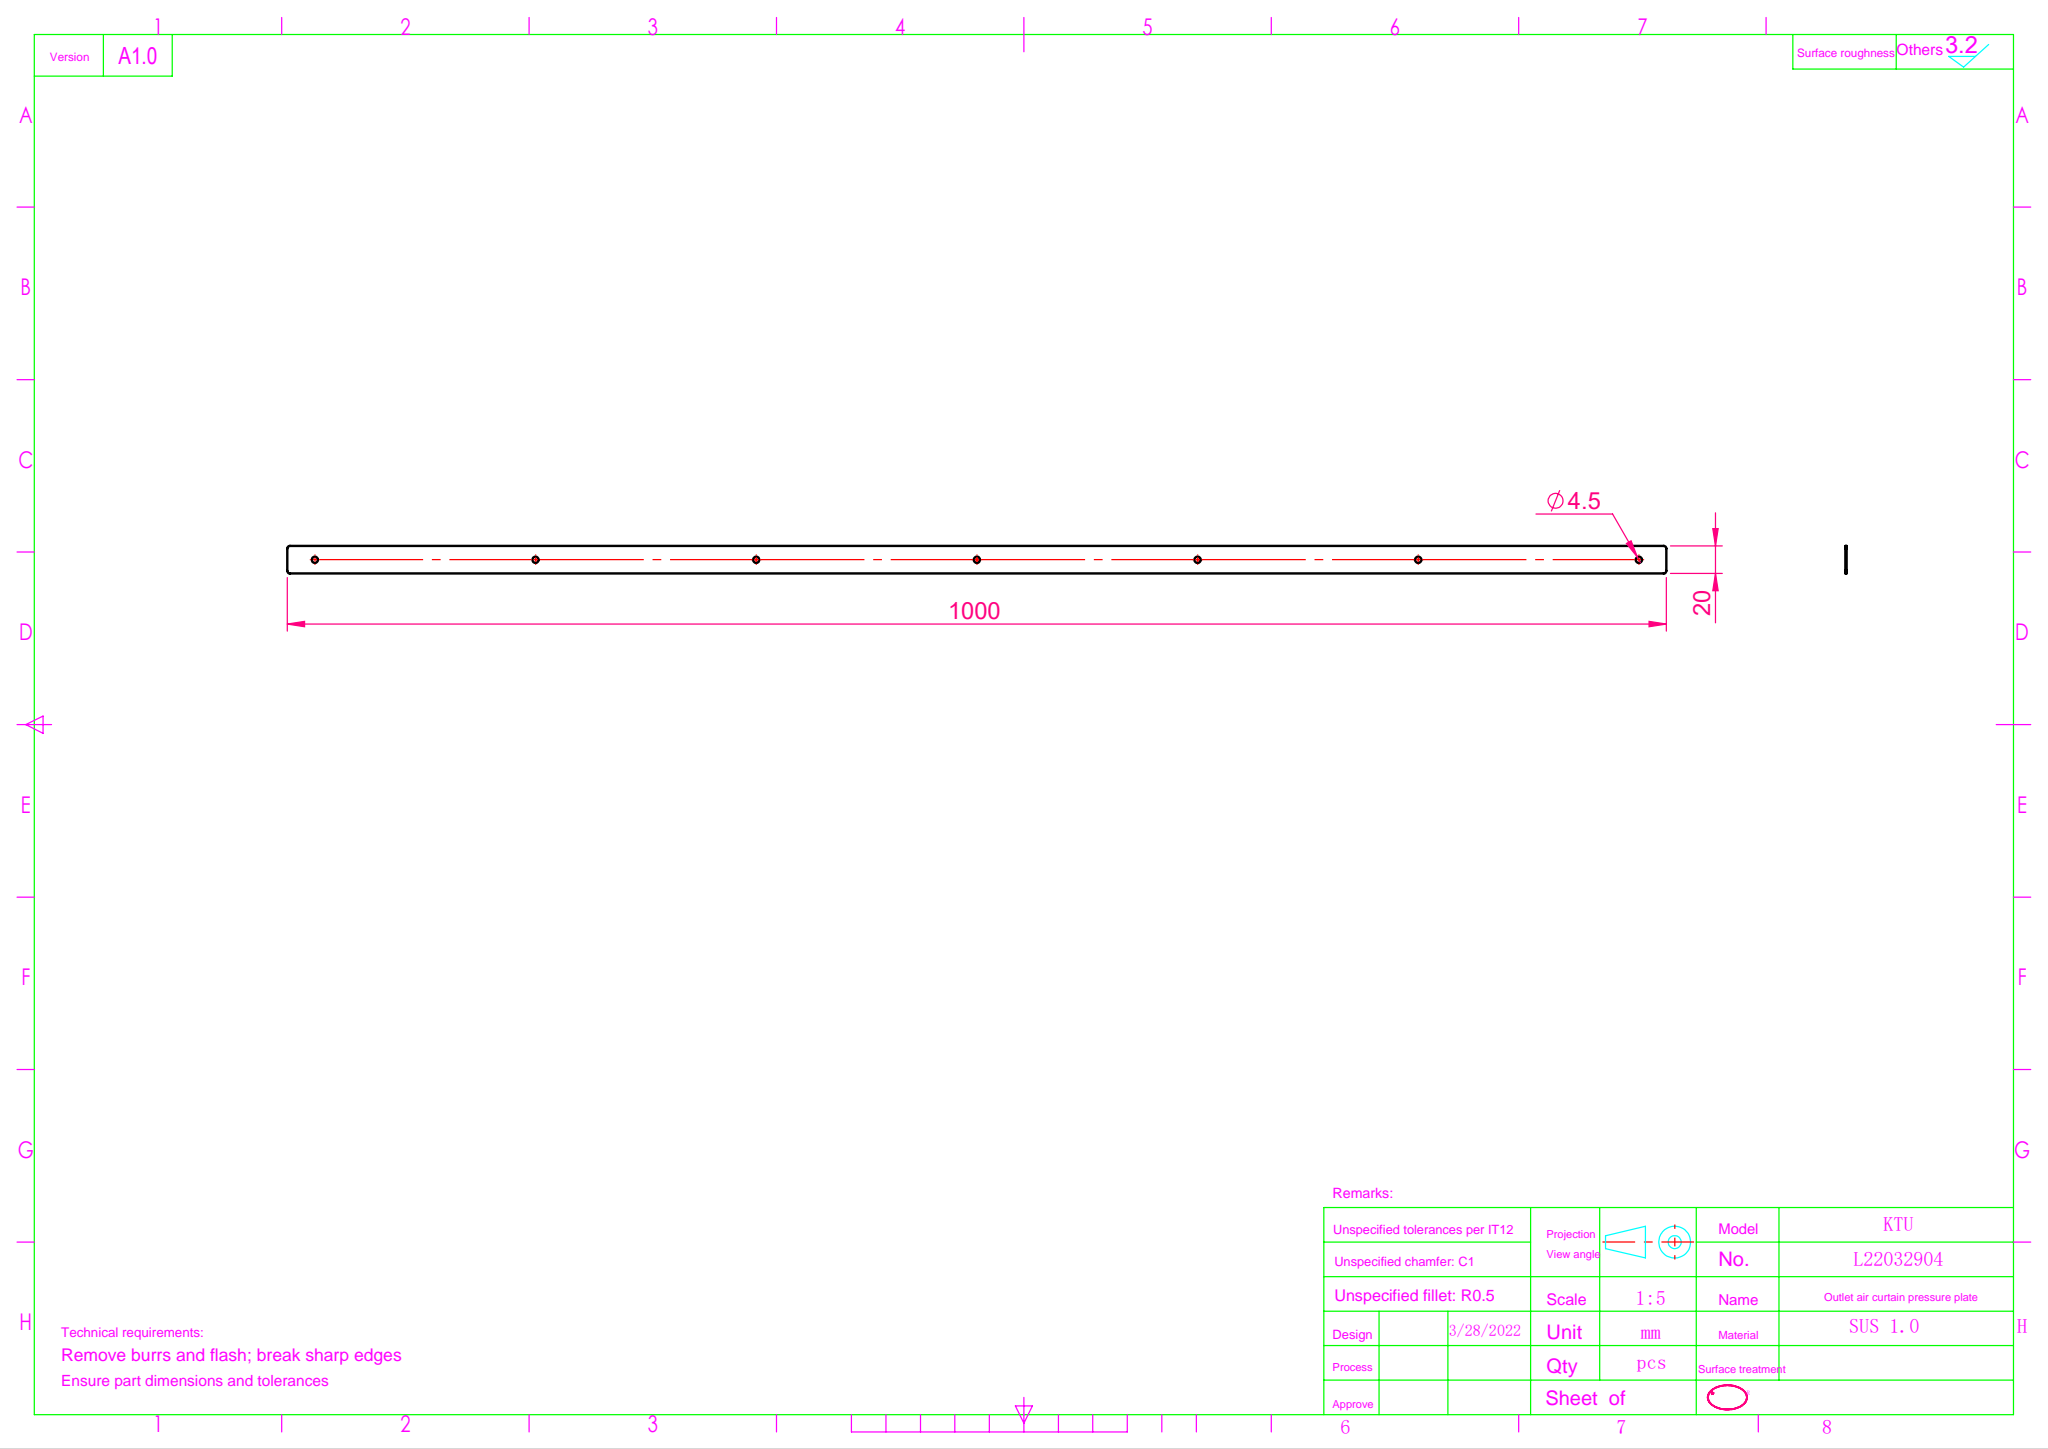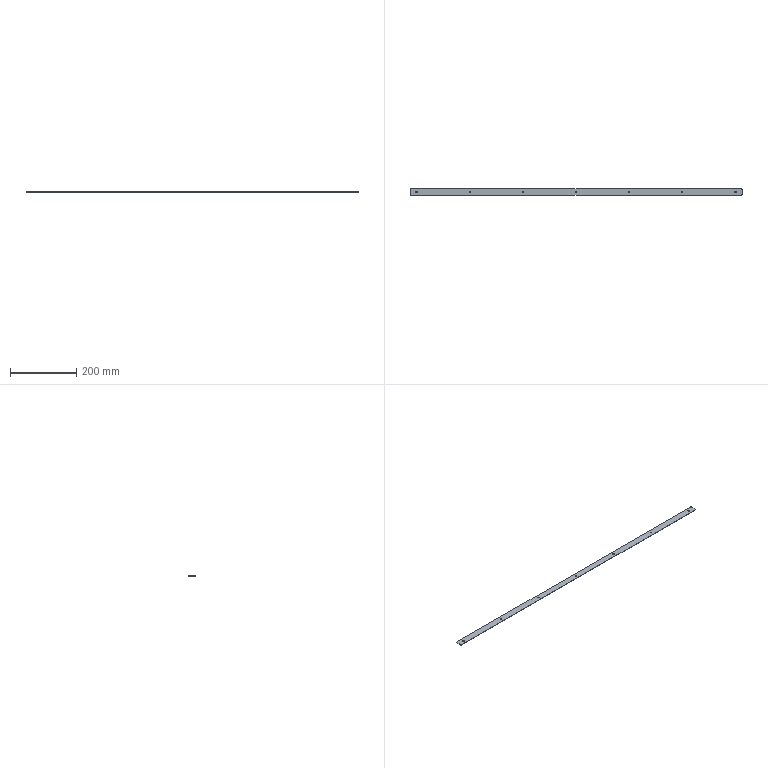Part | SolidWorks | features Fillet 1, FlatPattern 1, ICE 1, LPattern 1, SMBaseFlange 1, SheetMetal 1 | 1 solid | 24 faces | box 1000 x 20 x 1 mm | volume 19885 mm3 | cylinder 18 | plane 6 | commonest cylinder face diameters 4.5 x14 4 x4
STEP:
#1=CARTESIAN_POINT('',(-322.25,0.,-1.));
#2=VERTEX_POINT('',#1);
#3=CARTESIAN_POINT('',(-317.75,0.,-1.));
#4=VERTEX_POINT('',#3);
#5=CARTESIAN_POINT('',(-320.,0.,-1.));
#6=DIRECTION('',(0.,0.,1.));
#7=DIRECTION('',(1.,0.,0.));
#8=AXIS2_PLACEMENT_3D('',#5,#6,#7);
#9=CIRCLE('',#8,2.25);
#10=EDGE_CURVE('',#2,#4,#9,.T.);
#11=ORIENTED_EDGE('',*,*,#10,.F.);
#12=CARTESIAN_POINT('',(-322.25,0.,0.));
#13=VERTEX_POINT('',#12);
#14=CARTESIAN_POINT('',(-322.25,0.,-1.));
#15=DIRECTION('',(0.,0.,1.));
#16=VECTOR('',#15,1000.);
#17=LINE('',#14,#16);
#18=EDGE_CURVE('',#2,#13,#17,.T.);
#19=ORIENTED_EDGE('',*,*,#18,.T.);
#20=CARTESIAN_POINT('',(-317.75,0.,0.));
#21=VERTEX_POINT('',#20);
#22=CARTESIAN_POINT('',(-320.,0.,0.));
#23=DIRECTION('',(0.,0.,1.));
#24=DIRECTION('',(1.,0.,0.));
#25=AXIS2_PLACEMENT_3D('',#22,#23,#24);
#26=CIRCLE('',#25,2.25);
#27=EDGE_CURVE('',#13,#21,#26,.T.);
#28=ORIENTED_EDGE('',*,*,#27,.T.);
#29=CARTESIAN_POINT('',(-317.75,0.,-1.));
#30=DIRECTION('',(0.,0.,1.));
#31=VECTOR('',#30,1000.);
#32=LINE('',#29,#31);
#33=EDGE_CURVE('',#4,#21,#32,.T.);
#34=ORIENTED_EDGE('',*,*,#33,.F.);
#35=EDGE_LOOP('',(#11,#19,#28,#34));
#36=FACE_OUTER_BOUND('',#35,.T.);
#37=CARTESIAN_POINT('',(-320.,0.,-1.));
#38=DIRECTION('',(0.,0.,1.));
#39=DIRECTION('',(1.,0.,0.));
#40=AXIS2_PLACEMENT_3D('',#37,#38,#39);
#41=CYLINDRICAL_SURFACE('',#40,2.25);
#42=ADVANCED_FACE('',(#36),#41,.F.);
#43=CARTESIAN_POINT('',(317.75,0.,-1.));
#44=VERTEX_POINT('',#43);
#45=CARTESIAN_POINT('',(322.25,0.,-1.));
#46=VERTEX_POINT('',#45);
#47=CARTESIAN_POINT('',(320.,0.,-1.));
#48=DIRECTION('',(0.,0.,1.));
#49=DIRECTION('',(1.,0.,0.));
#50=AXIS2_PLACEMENT_3D('',#47,#48,#49);
#51=CIRCLE('',#50,2.25);
#52=EDGE_CURVE('',#44,#46,#51,.T.);
#53=ORIENTED_EDGE('',*,*,#52,.F.);
#54=CARTESIAN_POINT('',(317.75,0.,0.));
#55=VERTEX_POINT('',#54);
#56=CARTESIAN_POINT('',(317.75,0.,-1.));
#57=DIRECTION('',(0.,0.,1.));
#58=VECTOR('',#57,1000.);
#59=LINE('',#56,#58);
#60=EDGE_CURVE('',#44,#55,#59,.T.);
#61=ORIENTED_EDGE('',*,*,#60,.T.);
#62=CARTESIAN_POINT('',(322.25,0.,0.));
#63=VERTEX_POINT('',#62);
#64=CARTESIAN_POINT('',(320.,0.,0.));
#65=DIRECTION('',(0.,0.,1.));
#66=DIRECTION('',(1.,0.,0.));
#67=AXIS2_PLACEMENT_3D('',#64,#65,#66);
#68=CIRCLE('',#67,2.25);
#69=EDGE_CURVE('',#55,#63,#68,.T.);
#70=ORIENTED_EDGE('',*,*,#69,.T.);
#71=CARTESIAN_POINT('',(322.25,0.,-1.));
#72=DIRECTION('',(0.,0.,1.));
#73=VECTOR('',#72,1000.);
#74=LINE('',#71,#73);
#75=EDGE_CURVE('',#46,#63,#74,.T.);
#76=ORIENTED_EDGE('',*,*,#75,.F.);
#77=EDGE_LOOP('',(#53,#61,#70,#76));
#78=FACE_OUTER_BOUND('',#77,.T.);
#79=CARTESIAN_POINT('',(320.,0.,-1.));
#80=DIRECTION('',(0.,0.,1.));
#81=DIRECTION('',(1.,0.,0.));
#82=AXIS2_PLACEMENT_3D('',#79,#80,#81);
#83=CYLINDRICAL_SURFACE('',#82,2.25);
#84=ADVANCED_FACE('',(#78),#83,.F.);
#85=CARTESIAN_POINT('',(477.75,0.,-1.));
#86=VERTEX_POINT('',#85);
#87=CARTESIAN_POINT('',(482.25,0.,-1.));
#88=VERTEX_POINT('',#87);
#89=CARTESIAN_POINT('',(480.,0.,-1.));
#90=DIRECTION('',(0.,0.,1.));
#91=DIRECTION('',(1.,0.,0.));
#92=AXIS2_PLACEMENT_3D('',#89,#90,#91);
#93=CIRCLE('',#92,2.25);
#94=EDGE_CURVE('',#86,#88,#93,.T.);
#95=ORIENTED_EDGE('',*,*,#94,.F.);
#96=CARTESIAN_POINT('',(477.75,0.,0.));
#97=VERTEX_POINT('',#96);
#98=CARTESIAN_POINT('',(477.75,0.,-1.));
#99=DIRECTION('',(0.,0.,1.));
#100=VECTOR('',#99,1000.);
#101=LINE('',#98,#100);
#102=EDGE_CURVE('',#86,#97,#101,.T.);
#103=ORIENTED_EDGE('',*,*,#102,.T.);
#104=CARTESIAN_POINT('',(482.25,0.,0.));
#105=VERTEX_POINT('',#104);
#106=CARTESIAN_POINT('',(480.,0.,0.));
#107=DIRECTION('',(0.,0.,1.));
#108=DIRECTION('',(1.,0.,0.));
#109=AXIS2_PLACEMENT_3D('',#106,#107,#108);
#110=CIRCLE('',#109,2.25);
#111=EDGE_CURVE('',#97,#105,#110,.T.);
#112=ORIENTED_EDGE('',*,*,#111,.T.);
#113=CARTESIAN_POINT('',(482.25,0.,-1.));
#114=DIRECTION('',(0.,0.,1.));
#115=VECTOR('',#114,1000.);
#116=LINE('',#113,#115);
#117=EDGE_CURVE('',#88,#105,#116,.T.);
#118=ORIENTED_EDGE('',*,*,#117,.F.);
#119=EDGE_LOOP('',(#95,#103,#112,#118));
#120=FACE_OUTER_BOUND('',#119,.T.);
#121=CARTESIAN_POINT('',(480.,0.,-1.));
#122=DIRECTION('',(0.,0.,1.));
#123=DIRECTION('',(1.,0.,0.));
#124=AXIS2_PLACEMENT_3D('',#121,#122,#123);
#125=CYLINDRICAL_SURFACE('',#124,2.25);
#126=ADVANCED_FACE('',(#120),#125,.F.);
#127=CARTESIAN_POINT('',(-162.25,0.,-1.));
#128=VERTEX_POINT('',#127);
#129=CARTESIAN_POINT('',(-157.75,0.,-1.));
#130=VERTEX_POINT('',#129);
#131=CARTESIAN_POINT('',(-160.,0.,-1.));
#132=DIRECTION('',(0.,0.,1.));
#133=DIRECTION('',(1.,0.,0.));
#134=AXIS2_PLACEMENT_3D('',#131,#132,#133);
#135=CIRCLE('',#134,2.25);
#136=EDGE_CURVE('',#128,#130,#135,.T.);
#137=ORIENTED_EDGE('',*,*,#136,.F.);
#138=CARTESIAN_POINT('',(-162.25,0.,0.));
#139=VERTEX_POINT('',#138);
#140=CARTESIAN_POINT('',(-162.25,0.,-1.));
#141=DIRECTION('',(0.,0.,1.));
#142=VECTOR('',#141,1000.);
#143=LINE('',#140,#142);
#144=EDGE_CURVE('',#128,#139,#143,.T.);
#145=ORIENTED_EDGE('',*,*,#144,.T.);
#146=CARTESIAN_POINT('',(-157.75,0.,0.));
#147=VERTEX_POINT('',#146);
#148=CARTESIAN_POINT('',(-160.,0.,0.));
#149=DIRECTION('',(0.,0.,1.));
#150=DIRECTION('',(1.,0.,0.));
#151=AXIS2_PLACEMENT_3D('',#148,#149,#150);
#152=CIRCLE('',#151,2.25);
#153=EDGE_CURVE('',#139,#147,#152,.T.);
#154=ORIENTED_EDGE('',*,*,#153,.T.);
#155=CARTESIAN_POINT('',(-157.75,0.,-1.));
#156=DIRECTION('',(0.,0.,1.));
#157=VECTOR('',#156,1000.);
#158=LINE('',#155,#157);
#159=EDGE_CURVE('',#130,#147,#158,.T.);
#160=ORIENTED_EDGE('',*,*,#159,.F.);
#161=EDGE_LOOP('',(#137,#145,#154,#160));
#162=FACE_OUTER_BOUND('',#161,.T.);
#163=CARTESIAN_POINT('',(-160.,0.,-1.));
#164=DIRECTION('',(0.,0.,1.));
#165=DIRECTION('',(1.,0.,0.));
#166=AXIS2_PLACEMENT_3D('',#163,#164,#165);
#167=CYLINDRICAL_SURFACE('',#166,2.25);
#168=ADVANCED_FACE('',(#162),#167,.F.);
#169=CARTESIAN_POINT('',(-482.25,0.,-1.));
#170=VERTEX_POINT('',#169);
#171=CARTESIAN_POINT('',(-477.75,0.,-1.));
#172=VERTEX_POINT('',#171);
#173=CARTESIAN_POINT('',(-480.,0.,-1.));
#174=DIRECTION('',(0.,0.,1.));
#175=DIRECTION('',(1.,0.,0.));
#176=AXIS2_PLACEMENT_3D('',#173,#174,#175);
#177=CIRCLE('',#176,2.25);
#178=EDGE_CURVE('',#170,#172,#177,.T.);
#179=ORIENTED_EDGE('',*,*,#178,.F.);
#180=CARTESIAN_POINT('',(-482.25,0.,0.));
#181=VERTEX_POINT('',#180);
#182=CARTESIAN_POINT('',(-482.25,0.,-1.));
#183=DIRECTION('',(0.,0.,1.));
#184=VECTOR('',#183,1000.);
#185=LINE('',#182,#184);
#186=EDGE_CURVE('',#170,#181,#185,.T.);
#187=ORIENTED_EDGE('',*,*,#186,.T.);
#188=CARTESIAN_POINT('',(-477.75,0.,0.));
#189=VERTEX_POINT('',#188);
#190=CARTESIAN_POINT('',(-480.,0.,0.));
#191=DIRECTION('',(0.,0.,1.));
#192=DIRECTION('',(1.,0.,0.));
#193=AXIS2_PLACEMENT_3D('',#190,#191,#192);
#194=CIRCLE('',#193,2.25);
#195=EDGE_CURVE('',#181,#189,#194,.T.);
#196=ORIENTED_EDGE('',*,*,#195,.T.);
#197=CARTESIAN_POINT('',(-477.75,0.,-1.));
#198=DIRECTION('',(0.,0.,1.));
#199=VECTOR('',#198,1000.);
#200=LINE('',#197,#199);
#201=EDGE_CURVE('',#172,#189,#200,.T.);
#202=ORIENTED_EDGE('',*,*,#201,.F.);
#203=EDGE_LOOP('',(#179,#187,#196,#202));
#204=FACE_OUTER_BOUND('',#203,.T.);
#205=CARTESIAN_POINT('',(-480.,0.,-1.));
#206=DIRECTION('',(0.,0.,1.));
#207=DIRECTION('',(1.,0.,0.));
#208=AXIS2_PLACEMENT_3D('',#205,#206,#207);
#209=CYLINDRICAL_SURFACE('',#208,2.25);
#210=ADVANCED_FACE('',(#204),#209,.F.);
#211=CARTESIAN_POINT('',(157.75,0.,-1.));
#212=VERTEX_POINT('',#211);
#213=CARTESIAN_POINT('',(162.25,0.,-1.));
#214=VERTEX_POINT('',#213);
#215=CARTESIAN_POINT('',(160.,0.,-1.));
#216=DIRECTION('',(0.,0.,1.));
#217=DIRECTION('',(1.,0.,0.));
#218=AXIS2_PLACEMENT_3D('',#215,#216,#217);
#219=CIRCLE('',#218,2.25);
#220=EDGE_CURVE('',#212,#214,#219,.T.);
#221=ORIENTED_EDGE('',*,*,#220,.F.);
#222=CARTESIAN_POINT('',(157.75,0.,0.));
#223=VERTEX_POINT('',#222);
#224=CARTESIAN_POINT('',(157.75,0.,-1.));
#225=DIRECTION('',(0.,0.,1.));
#226=VECTOR('',#225,1000.);
#227=LINE('',#224,#226);
#228=EDGE_CURVE('',#212,#223,#227,.T.);
#229=ORIENTED_EDGE('',*,*,#228,.T.);
#230=CARTESIAN_POINT('',(162.25,0.,0.));
#231=VERTEX_POINT('',#230);
#232=CARTESIAN_POINT('',(160.,0.,0.));
#233=DIRECTION('',(0.,0.,1.));
#234=DIRECTION('',(1.,0.,0.));
#235=AXIS2_PLACEMENT_3D('',#232,#233,#234);
#236=CIRCLE('',#235,2.25);
#237=EDGE_CURVE('',#223,#231,#236,.T.);
#238=ORIENTED_EDGE('',*,*,#237,.T.);
#239=CARTESIAN_POINT('',(162.25,0.,-1.));
#240=DIRECTION('',(0.,0.,1.));
#241=VECTOR('',#240,1000.);
#242=LINE('',#239,#241);
#243=EDGE_CURVE('',#214,#231,#242,.T.);
#244=ORIENTED_EDGE('',*,*,#243,.F.);
#245=EDGE_LOOP('',(#221,#229,#238,#244));
#246=FACE_OUTER_BOUND('',#245,.T.);
#247=CARTESIAN_POINT('',(160.,0.,-1.));
#248=DIRECTION('',(0.,0.,1.));
#249=DIRECTION('',(1.,0.,0.));
#250=AXIS2_PLACEMENT_3D('',#247,#248,#249);
#251=CYLINDRICAL_SURFACE('',#250,2.25);
#252=ADVANCED_FACE('',(#246),#251,.F.);
#253=CARTESIAN_POINT('',(-2.25,0.,-1.));
#254=VERTEX_POINT('',#253);
#255=CARTESIAN_POINT('',(2.25,0.,-1.));
#256=VERTEX_POINT('',#255);
#257=CARTESIAN_POINT('',(0.,0.,-1.));
#258=DIRECTION('',(0.,0.,1.));
#259=DIRECTION('',(1.,0.,0.));
#260=AXIS2_PLACEMENT_3D('',#257,#258,#259);
#261=CIRCLE('',#260,2.25);
#262=EDGE_CURVE('',#254,#256,#261,.T.);
#263=ORIENTED_EDGE('',*,*,#262,.F.);
#264=CARTESIAN_POINT('',(-2.25,0.,0.));
#265=VERTEX_POINT('',#264);
#266=CARTESIAN_POINT('',(-2.25,0.,-1.));
#267=DIRECTION('',(0.,0.,1.));
#268=VECTOR('',#267,1000.);
#269=LINE('',#266,#268);
#270=EDGE_CURVE('',#254,#265,#269,.T.);
#271=ORIENTED_EDGE('',*,*,#270,.T.);
#272=CARTESIAN_POINT('',(2.25,0.,0.));
#273=VERTEX_POINT('',#272);
#274=CARTESIAN_POINT('',(0.,0.,0.));
#275=DIRECTION('',(0.,0.,1.));
#276=DIRECTION('',(1.,0.,0.));
#277=AXIS2_PLACEMENT_3D('',#274,#275,#276);
#278=CIRCLE('',#277,2.25);
#279=EDGE_CURVE('',#265,#273,#278,.T.);
#280=ORIENTED_EDGE('',*,*,#279,.T.);
#281=CARTESIAN_POINT('',(2.25,0.,-1.));
#282=DIRECTION('',(0.,0.,1.));
#283=VECTOR('',#282,1000.);
#284=LINE('',#281,#283);
#285=EDGE_CURVE('',#256,#273,#284,.T.);
#286=ORIENTED_EDGE('',*,*,#285,.F.);
#287=EDGE_LOOP('',(#263,#271,#280,#286));
#288=FACE_OUTER_BOUND('',#287,.T.);
#289=CARTESIAN_POINT('',(0.,0.,-1.));
#290=DIRECTION('',(0.,0.,1.));
#291=DIRECTION('',(1.,0.,0.));
#292=AXIS2_PLACEMENT_3D('',#289,#290,#291);
#293=CYLINDRICAL_SURFACE('',#292,2.25);
#294=ADVANCED_FACE('',(#288),#293,.F.);
#295=CARTESIAN_POINT('',(500.,-8.,0.));
#296=VERTEX_POINT('',#295);
#297=CARTESIAN_POINT('',(500.,8.,0.));
#298=VERTEX_POINT('',#297);
#299=CARTESIAN_POINT('',(500.,10.,0.));
#300=DIRECTION('',(0.,1.,0.));
#301=VECTOR('',#300,1000.);
#302=LINE('',#299,#301);
#303=EDGE_CURVE('',#296,#298,#302,.T.);
#304=ORIENTED_EDGE('',*,*,#303,.F.);
#305=CARTESIAN_POINT('',(500.,-8.,-1.));
#306=VERTEX_POINT('',#305);
#307=CARTESIAN_POINT('',(500.,-8.,-1.));
#308=DIRECTION('',(0.,0.,-1.));
#309=VECTOR('',#308,1000.);
#310=LINE('',#307,#309);
#311=EDGE_CURVE('',#296,#306,#310,.T.);
#312=ORIENTED_EDGE('',*,*,#311,.T.);
#313=CARTESIAN_POINT('',(500.,8.,-1.));
#314=VERTEX_POINT('',#313);
#315=CARTESIAN_POINT('',(500.,10.,-1.));
#316=DIRECTION('',(0.,1.,0.));
#317=VECTOR('',#316,1000.);
#318=LINE('',#315,#317);
#319=EDGE_CURVE('',#306,#314,#318,.T.);
#320=ORIENTED_EDGE('',*,*,#319,.T.);
#321=CARTESIAN_POINT('',(500.,8.,-1.));
#322=DIRECTION('',(0.,0.,1.));
#323=VECTOR('',#322,1000.);
#324=LINE('',#321,#323);
#325=EDGE_CURVE('',#314,#298,#324,.T.);
#326=ORIENTED_EDGE('',*,*,#325,.T.);
#327=EDGE_LOOP('',(#304,#312,#320,#326));
#328=FACE_OUTER_BOUND('',#327,.T.);
#329=CARTESIAN_POINT('',(500.,10.,-1.));
#330=DIRECTION('',(1.,0.,0.));
#331=DIRECTION('',(0.,0.,-1.));
#332=AXIS2_PLACEMENT_3D('',#329,#330,#331);
#333=PLANE('',#332);
#334=ADVANCED_FACE('',(#328),#333,.T.);
#335=CARTESIAN_POINT('',(-498.,-10.,-1.));
#336=VERTEX_POINT('',#335);
#337=CARTESIAN_POINT('',(498.,-10.,-1.));
#338=VERTEX_POINT('',#337);
#339=CARTESIAN_POINT('',(-500.,-10.,-1.));
#340=DIRECTION('',(1.,0.,0.));
#341=VECTOR('',#340,1000.);
#342=LINE('',#339,#341);
#343=EDGE_CURVE('',#336,#338,#342,.T.);
#344=ORIENTED_EDGE('',*,*,#343,.T.);
#345=CARTESIAN_POINT('',(498.,-10.,0.));
#346=VERTEX_POINT('',#345);
#347=CARTESIAN_POINT('',(498.,-10.,-1.));
#348=DIRECTION('',(0.,0.,1.));
#349=VECTOR('',#348,1000.);
#350=LINE('',#347,#349);
#351=EDGE_CURVE('',#338,#346,#350,.T.);
#352=ORIENTED_EDGE('',*,*,#351,.T.);
#353=CARTESIAN_POINT('',(-498.,-10.,0.));
#354=VERTEX_POINT('',#353);
#355=CARTESIAN_POINT('',(-500.,-10.,0.));
#356=DIRECTION('',(1.,0.,0.));
#357=VECTOR('',#356,1000.);
#358=LINE('',#355,#357);
#359=EDGE_CURVE('',#354,#346,#358,.T.);
#360=ORIENTED_EDGE('',*,*,#359,.F.);
#361=CARTESIAN_POINT('',(-498.,-10.,-1.));
#362=DIRECTION('',(0.,0.,-1.));
#363=VECTOR('',#362,1000.);
#364=LINE('',#361,#363);
#365=EDGE_CURVE('',#354,#336,#364,.T.);
#366=ORIENTED_EDGE('',*,*,#365,.T.);
#367=EDGE_LOOP('',(#344,#352,#360,#366));
#368=FACE_OUTER_BOUND('',#367,.T.);
#369=CARTESIAN_POINT('',(-500.,-10.,-1.));
#370=DIRECTION('',(0.,-1.,0.));
#371=DIRECTION('',(0.,0.,-1.));
#372=AXIS2_PLACEMENT_3D('',#369,#370,#371);
#373=PLANE('',#372);
#374=ADVANCED_FACE('',(#368),#373,.T.);
#375=CARTESIAN_POINT('',(-500.,8.,-1.));
#376=VERTEX_POINT('',#375);
#377=CARTESIAN_POINT('',(-500.,-8.,-1.));
#378=VERTEX_POINT('',#377);
#379=CARTESIAN_POINT('',(-500.,10.,-1.));
#380=DIRECTION('',(0.,-1.,0.));
#381=VECTOR('',#380,1000.);
#382=LINE('',#379,#381);
#383=EDGE_CURVE('',#376,#378,#382,.T.);
#384=ORIENTED_EDGE('',*,*,#383,.T.);
#385=CARTESIAN_POINT('',(-500.,-8.,0.));
#386=VERTEX_POINT('',#385);
#387=CARTESIAN_POINT('',(-500.,-8.,-1.));
#388=DIRECTION('',(0.,0.,1.));
#389=VECTOR('',#388,1000.);
#390=LINE('',#387,#389);
#391=EDGE_CURVE('',#378,#386,#390,.T.);
#392=ORIENTED_EDGE('',*,*,#391,.T.);
#393=CARTESIAN_POINT('',(-500.,8.,0.));
#394=VERTEX_POINT('',#393);
#395=CARTESIAN_POINT('',(-500.,10.,0.));
#396=DIRECTION('',(0.,-1.,0.));
#397=VECTOR('',#396,1000.);
#398=LINE('',#395,#397);
#399=EDGE_CURVE('',#394,#386,#398,.T.);
#400=ORIENTED_EDGE('',*,*,#399,.F.);
#401=CARTESIAN_POINT('',(-500.,8.,-1.));
#402=DIRECTION('',(0.,0.,-1.));
#403=VECTOR('',#402,1000.);
#404=LINE('',#401,#403);
#405=EDGE_CURVE('',#394,#376,#404,.T.);
#406=ORIENTED_EDGE('',*,*,#405,.T.);
#407=EDGE_LOOP('',(#384,#392,#400,#406));
#408=FACE_OUTER_BOUND('',#407,.T.);
#409=CARTESIAN_POINT('',(-500.,10.,-1.));
#410=DIRECTION('',(-1.,0.,0.));
#411=DIRECTION('',(0.,0.,1.));
#412=AXIS2_PLACEMENT_3D('',#409,#410,#411);
#413=PLANE('',#412);
#414=ADVANCED_FACE('',(#408),#413,.T.);
#415=CARTESIAN_POINT('',(498.,10.,0.));
#416=VERTEX_POINT('',#415);
#417=CARTESIAN_POINT('',(-498.,10.,0.));
#418=VERTEX_POINT('',#417);
#419=CARTESIAN_POINT('',(-500.,10.,0.));
#420=DIRECTION('',(-1.,0.,0.));
#421=VECTOR('',#420,1000.);
#422=LINE('',#419,#421);
#423=EDGE_CURVE('',#416,#418,#422,.T.);
#424=ORIENTED_EDGE('',*,*,#423,.F.);
#425=CARTESIAN_POINT('',(498.,10.,-1.));
#426=VERTEX_POINT('',#425);
#427=CARTESIAN_POINT('',(498.,10.,-1.));
#428=DIRECTION('',(0.,0.,-1.));
#429=VECTOR('',#428,1000.);
#430=LINE('',#427,#429);
#431=EDGE_CURVE('',#416,#426,#430,.T.);
#432=ORIENTED_EDGE('',*,*,#431,.T.);
#433=CARTESIAN_POINT('',(-498.,10.,-1.));
#434=VERTEX_POINT('',#433);
#435=CARTESIAN_POINT('',(-500.,10.,-1.));
#436=DIRECTION('',(-1.,0.,0.));
#437=VECTOR('',#436,1000.);
#438=LINE('',#435,#437);
#439=EDGE_CURVE('',#426,#434,#438,.T.);
#440=ORIENTED_EDGE('',*,*,#439,.T.);
#441=CARTESIAN_POINT('',(-498.,10.,-1.));
#442=DIRECTION('',(0.,0.,1.));
#443=VECTOR('',#442,1000.);
#444=LINE('',#441,#443);
#445=EDGE_CURVE('',#434,#418,#444,.T.);
#446=ORIENTED_EDGE('',*,*,#445,.T.);
#447=EDGE_LOOP('',(#424,#432,#440,#446));
#448=FACE_OUTER_BOUND('',#447,.T.);
#449=CARTESIAN_POINT('',(-500.,10.,-1.));
#450=DIRECTION('',(0.,1.,0.));
#451=DIRECTION('',(0.,0.,1.));
#452=AXIS2_PLACEMENT_3D('',#449,#450,#451);
#453=PLANE('',#452);
#454=ADVANCED_FACE('',(#448),#453,.T.);
#455=CARTESIAN_POINT('',(-320.,0.,-1.));
#456=DIRECTION('',(0.,0.,1.));
#457=DIRECTION('',(1.,0.,0.));
#458=AXIS2_PLACEMENT_3D('',#455,#456,#457);
#459=CIRCLE('',#458,2.25);
#460=EDGE_CURVE('',#4,#2,#459,.T.);
#461=ORIENTED_EDGE('',*,*,#460,.T.);
#462=ORIENTED_EDGE('',*,*,#10,.T.);
#463=EDGE_LOOP('',(#461,#462));
#464=FACE_BOUND('',#463,.T.);
#465=CARTESIAN_POINT('',(320.,0.,-1.));
#466=DIRECTION('',(0.,0.,1.));
#467=DIRECTION('',(1.,0.,0.));
#468=AXIS2_PLACEMENT_3D('',#465,#466,#467);
#469=CIRCLE('',#468,2.25);
#470=EDGE_CURVE('',#46,#44,#469,.T.);
#471=ORIENTED_EDGE('',*,*,#470,.T.);
#472=ORIENTED_EDGE('',*,*,#52,.T.);
#473=EDGE_LOOP('',(#471,#472));
#474=FACE_BOUND('',#473,.T.);
#475=CARTESIAN_POINT('',(480.,0.,-1.));
#476=DIRECTION('',(0.,0.,1.));
#477=DIRECTION('',(1.,0.,0.));
#478=AXIS2_PLACEMENT_3D('',#475,#476,#477);
#479=CIRCLE('',#478,2.25);
#480=EDGE_CURVE('',#88,#86,#479,.T.);
#481=ORIENTED_EDGE('',*,*,#480,.T.);
#482=ORIENTED_EDGE('',*,*,#94,.T.);
#483=EDGE_LOOP('',(#481,#482));
#484=FACE_BOUND('',#483,.T.);
#485=CARTESIAN_POINT('',(-160.,0.,-1.));
#486=DIRECTION('',(0.,0.,1.));
#487=DIRECTION('',(1.,0.,0.));
#488=AXIS2_PLACEMENT_3D('',#485,#486,#487);
#489=CIRCLE('',#488,2.25);
#490=EDGE_CURVE('',#130,#128,#489,.T.);
#491=ORIENTED_EDGE('',*,*,#490,.T.);
#492=ORIENTED_EDGE('',*,*,#136,.T.);
#493=EDGE_LOOP('',(#491,#492));
#494=FACE_BOUND('',#493,.T.);
#495=CARTESIAN_POINT('',(-480.,0.,-1.));
#496=DIRECTION('',(0.,0.,1.));
#497=DIRECTION('',(1.,0.,0.));
#498=AXIS2_PLACEMENT_3D('',#495,#496,#497);
#499=CIRCLE('',#498,2.25);
#500=EDGE_CURVE('',#172,#170,#499,.T.);
#501=ORIENTED_EDGE('',*,*,#500,.T.);
#502=ORIENTED_EDGE('',*,*,#178,.T.);
#503=EDGE_LOOP('',(#501,#502));
#504=FACE_BOUND('',#503,.T.);
#505=CARTESIAN_POINT('',(160.,0.,-1.));
#506=DIRECTION('',(0.,0.,1.));
#507=DIRECTION('',(1.,0.,0.));
#508=AXIS2_PLACEMENT_3D('',#505,#506,#507);
#509=CIRCLE('',#508,2.25);
#510=EDGE_CURVE('',#214,#212,#509,.T.);
#511=ORIENTED_EDGE('',*,*,#510,.T.);
#512=ORIENTED_EDGE('',*,*,#220,.T.);
#513=EDGE_LOOP('',(#511,#512));
#514=FACE_BOUND('',#513,.T.);
#515=CARTESIAN_POINT('',(0.,0.,-1.));
#516=DIRECTION('',(0.,0.,1.));
#517=DIRECTION('',(1.,0.,0.));
#518=AXIS2_PLACEMENT_3D('',#515,#516,#517);
#519=CIRCLE('',#518,2.25);
#520=EDGE_CURVE('',#256,#254,#519,.T.);
#521=ORIENTED_EDGE('',*,*,#520,.T.);
#522=ORIENTED_EDGE('',*,*,#262,.T.);
#523=EDGE_LOOP('',(#521,#522));
#524=FACE_BOUND('',#523,.T.);
#525=ORIENTED_EDGE('',*,*,#319,.F.);
#526=CARTESIAN_POINT('',(498.,-8.,-1.));
#527=DIRECTION('',(0.,0.,-1.));
#528=DIRECTION('',(1.,0.,0.));
#529=AXIS2_PLACEMENT_3D('',#526,#527,#528);
#530=CIRCLE('',#529,2.);
#531=EDGE_CURVE('',#306,#338,#530,.T.);
#532=ORIENTED_EDGE('',*,*,#531,.T.);
#533=ORIENTED_EDGE('',*,*,#343,.F.);
#534=CARTESIAN_POINT('',(-498.,-8.,-1.));
#535=DIRECTION('',(0.,0.,-1.));
#536=DIRECTION('',(1.,0.,0.));
#537=AXIS2_PLACEMENT_3D('',#534,#535,#536);
#538=CIRCLE('',#537,2.);
#539=EDGE_CURVE('',#336,#378,#538,.T.);
#540=ORIENTED_EDGE('',*,*,#539,.T.);
#541=ORIENTED_EDGE('',*,*,#383,.F.);
#542=CARTESIAN_POINT('',(-498.,8.,-1.));
#543=DIRECTION('',(0.,0.,-1.));
#544=DIRECTION('',(1.,0.,0.));
#545=AXIS2_PLACEMENT_3D('',#542,#543,#544);
#546=CIRCLE('',#545,2.);
#547=EDGE_CURVE('',#376,#434,#546,.T.);
#548=ORIENTED_EDGE('',*,*,#547,.T.);
#549=ORIENTED_EDGE('',*,*,#439,.F.);
#550=CARTESIAN_POINT('',(498.,8.,-1.));
#551=DIRECTION('',(0.,0.,-1.));
#552=DIRECTION('',(1.,0.,0.));
#553=AXIS2_PLACEMENT_3D('',#550,#551,#552);
#554=CIRCLE('',#553,2.);
#555=EDGE_CURVE('',#426,#314,#554,.T.);
#556=ORIENTED_EDGE('',*,*,#555,.T.);
#557=EDGE_LOOP('',(#525,#532,#533,#540,#541,#548,#549,#556));
#558=FACE_OUTER_BOUND('',#557,.T.);
#559=CARTESIAN_POINT('',(0.,0.,-1.));
#560=DIRECTION('',(0.,0.,1.));
#561=DIRECTION('',(1.,0.,0.));
#562=AXIS2_PLACEMENT_3D('',#559,#560,#561);
#563=PLANE('',#562);
#564=ADVANCED_FACE('',(#464,#474,#484,#494,#504,#514,#524,#558),#563,.F.);
#565=CARTESIAN_POINT('',(-320.,0.,0.));
#566=DIRECTION('',(0.,0.,1.));
#567=DIRECTION('',(1.,0.,0.));
#568=AXIS2_PLACEMENT_3D('',#565,#566,#567);
#569=CIRCLE('',#568,2.25);
#570=EDGE_CURVE('',#21,#13,#569,.T.);
#571=ORIENTED_EDGE('',*,*,#570,.F.);
#572=ORIENTED_EDGE('',*,*,#27,.F.);
#573=EDGE_LOOP('',(#571,#572));
#574=FACE_BOUND('',#573,.T.);
#575=CARTESIAN_POINT('',(320.,0.,0.));
#576=DIRECTION('',(0.,0.,1.));
#577=DIRECTION('',(1.,0.,0.));
#578=AXIS2_PLACEMENT_3D('',#575,#576,#577);
#579=CIRCLE('',#578,2.25);
#580=EDGE_CURVE('',#63,#55,#579,.T.);
#581=ORIENTED_EDGE('',*,*,#580,.F.);
#582=ORIENTED_EDGE('',*,*,#69,.F.);
#583=EDGE_LOOP('',(#581,#582));
#584=FACE_BOUND('',#583,.T.);
#585=CARTESIAN_POINT('',(480.,0.,0.));
#586=DIRECTION('',(0.,0.,1.));
#587=DIRECTION('',(1.,0.,0.));
#588=AXIS2_PLACEMENT_3D('',#585,#586,#587);
#589=CIRCLE('',#588,2.25);
#590=EDGE_CURVE('',#105,#97,#589,.T.);
#591=ORIENTED_EDGE('',*,*,#590,.F.);
#592=ORIENTED_EDGE('',*,*,#111,.F.);
#593=EDGE_LOOP('',(#591,#592));
#594=FACE_BOUND('',#593,.T.);
#595=CARTESIAN_POINT('',(-160.,0.,0.));
#596=DIRECTION('',(0.,0.,1.));
#597=DIRECTION('',(1.,0.,0.));
#598=AXIS2_PLACEMENT_3D('',#595,#596,#597);
#599=CIRCLE('',#598,2.25);
#600=EDGE_CURVE('',#147,#139,#599,.T.);
#601=ORIENTED_EDGE('',*,*,#600,.F.);
#602=ORIENTED_EDGE('',*,*,#153,.F.);
#603=EDGE_LOOP('',(#601,#602));
#604=FACE_BOUND('',#603,.T.);
#605=CARTESIAN_POINT('',(-480.,0.,0.));
#606=DIRECTION('',(0.,0.,1.));
#607=DIRECTION('',(1.,0.,0.));
#608=AXIS2_PLACEMENT_3D('',#605,#606,#607);
#609=CIRCLE('',#608,2.25);
#610=EDGE_CURVE('',#189,#181,#609,.T.);
#611=ORIENTED_EDGE('',*,*,#610,.F.);
#612=ORIENTED_EDGE('',*,*,#195,.F.);
#613=EDGE_LOOP('',(#611,#612));
#614=FACE_BOUND('',#613,.T.);
#615=CARTESIAN_POINT('',(160.,0.,0.));
#616=DIRECTION('',(0.,0.,1.));
#617=DIRECTION('',(1.,0.,0.));
#618=AXIS2_PLACEMENT_3D('',#615,#616,#617);
#619=CIRCLE('',#618,2.25);
#620=EDGE_CURVE('',#231,#223,#619,.T.);
#621=ORIENTED_EDGE('',*,*,#620,.F.);
#622=ORIENTED_EDGE('',*,*,#237,.F.);
#623=EDGE_LOOP('',(#621,#622));
#624=FACE_BOUND('',#623,.T.);
#625=CARTESIAN_POINT('',(0.,0.,0.));
#626=DIRECTION('',(0.,0.,1.));
#627=DIRECTION('',(1.,0.,0.));
#628=AXIS2_PLACEMENT_3D('',#625,#626,#627);
#629=CIRCLE('',#628,2.25);
#630=EDGE_CURVE('',#273,#265,#629,.T.);
#631=ORIENTED_EDGE('',*,*,#630,.F.);
#632=ORIENTED_EDGE('',*,*,#279,.F.);
#633=EDGE_LOOP('',(#631,#632));
#634=FACE_BOUND('',#633,.T.);
#635=ORIENTED_EDGE('',*,*,#359,.T.);
#636=CARTESIAN_POINT('',(498.,-8.,0.));
#637=DIRECTION('',(0.,0.,1.));
#638=DIRECTION('',(1.,0.,0.));
#639=AXIS2_PLACEMENT_3D('',#636,#637,#638);
#640=CIRCLE('',#639,2.);
#641=EDGE_CURVE('',#346,#296,#640,.T.);
#642=ORIENTED_EDGE('',*,*,#641,.T.);
#643=ORIENTED_EDGE('',*,*,#303,.T.);
#644=CARTESIAN_POINT('',(498.,8.,0.));
#645=DIRECTION('',(0.,0.,1.));
#646=DIRECTION('',(1.,0.,0.));
#647=AXIS2_PLACEMENT_3D('',#644,#645,#646);
#648=CIRCLE('',#647,2.);
#649=EDGE_CURVE('',#298,#416,#648,.T.);
#650=ORIENTED_EDGE('',*,*,#649,.T.);
#651=ORIENTED_EDGE('',*,*,#423,.T.);
#652=CARTESIAN_POINT('',(-498.,8.,0.));
#653=DIRECTION('',(0.,0.,1.));
#654=DIRECTION('',(1.,0.,0.));
#655=AXIS2_PLACEMENT_3D('',#652,#653,#654);
#656=CIRCLE('',#655,2.);
#657=EDGE_CURVE('',#418,#394,#656,.T.);
#658=ORIENTED_EDGE('',*,*,#657,.T.);
#659=ORIENTED_EDGE('',*,*,#399,.T.);
#660=CARTESIAN_POINT('',(-498.,-8.,0.));
#661=DIRECTION('',(0.,0.,1.));
#662=DIRECTION('',(1.,0.,0.));
#663=AXIS2_PLACEMENT_3D('',#660,#661,#662);
#664=CIRCLE('',#663,2.);
#665=EDGE_CURVE('',#386,#354,#664,.T.);
#666=ORIENTED_EDGE('',*,*,#665,.T.);
#667=EDGE_LOOP('',(#635,#642,#643,#650,#651,#658,#659,#666));
#668=FACE_OUTER_BOUND('',#667,.T.);
#669=CARTESIAN_POINT('',(0.,0.,0.));
#670=DIRECTION('',(0.,0.,1.));
#671=DIRECTION('',(1.,0.,0.));
#672=AXIS2_PLACEMENT_3D('',#669,#670,#671);
#673=PLANE('',#672);
#674=ADVANCED_FACE('',(#574,#584,#594,#604,#614,#624,#634,#668),#673,.T.);
#675=ORIENTED_EDGE('',*,*,#270,.F.);
#676=ORIENTED_EDGE('',*,*,#520,.F.);
#677=ORIENTED_EDGE('',*,*,#285,.T.);
#678=ORIENTED_EDGE('',*,*,#630,.T.);
#679=EDGE_LOOP('',(#675,#676,#677,#678));
#680=FACE_OUTER_BOUND('',#679,.T.);
#681=CARTESIAN_POINT('',(0.,0.,-1.));
#682=DIRECTION('',(0.,0.,1.));
#683=DIRECTION('',(1.,0.,0.));
#684=AXIS2_PLACEMENT_3D('',#681,#682,#683);
#685=CYLINDRICAL_SURFACE('',#684,2.25);
#686=ADVANCED_FACE('',(#680),#685,.F.);
#687=ORIENTED_EDGE('',*,*,#228,.F.);
#688=ORIENTED_EDGE('',*,*,#510,.F.);
#689=ORIENTED_EDGE('',*,*,#243,.T.);
#690=ORIENTED_EDGE('',*,*,#620,.T.);
#691=EDGE_LOOP('',(#687,#688,#689,#690));
#692=FACE_OUTER_BOUND('',#691,.T.);
#693=CARTESIAN_POINT('',(160.,0.,-1.));
#694=DIRECTION('',(0.,0.,1.));
#695=DIRECTION('',(1.,0.,0.));
#696=AXIS2_PLACEMENT_3D('',#693,#694,#695);
#697=CYLINDRICAL_SURFACE('',#696,2.25);
#698=ADVANCED_FACE('',(#692),#697,.F.);
#699=ORIENTED_EDGE('',*,*,#186,.F.);
#700=ORIENTED_EDGE('',*,*,#500,.F.);
#701=ORIENTED_EDGE('',*,*,#201,.T.);
#702=ORIENTED_EDGE('',*,*,#610,.T.);
#703=EDGE_LOOP('',(#699,#700,#701,#702));
#704=FACE_OUTER_BOUND('',#703,.T.);
#705=CARTESIAN_POINT('',(-480.,0.,-1.));
#706=DIRECTION('',(0.,0.,1.));
#707=DIRECTION('',(1.,0.,0.));
#708=AXIS2_PLACEMENT_3D('',#705,#706,#707);
#709=CYLINDRICAL_SURFACE('',#708,2.25);
#710=ADVANCED_FACE('',(#704),#709,.F.);
#711=ORIENTED_EDGE('',*,*,#144,.F.);
#712=ORIENTED_EDGE('',*,*,#490,.F.);
#713=ORIENTED_EDGE('',*,*,#159,.T.);
#714=ORIENTED_EDGE('',*,*,#600,.T.);
#715=EDGE_LOOP('',(#711,#712,#713,#714));
#716=FACE_OUTER_BOUND('',#715,.T.);
#717=CARTESIAN_POINT('',(-160.,0.,-1.));
#718=DIRECTION('',(0.,0.,1.));
#719=DIRECTION('',(1.,0.,0.));
#720=AXIS2_PLACEMENT_3D('',#717,#718,#719);
#721=CYLINDRICAL_SURFACE('',#720,2.25);
#722=ADVANCED_FACE('',(#716),#721,.F.);
#723=ORIENTED_EDGE('',*,*,#102,.F.);
#724=ORIENTED_EDGE('',*,*,#480,.F.);
#725=ORIENTED_EDGE('',*,*,#117,.T.);
#726=ORIENTED_EDGE('',*,*,#590,.T.);
#727=EDGE_LOOP('',(#723,#724,#725,#726));
#728=FACE_OUTER_BOUND('',#727,.T.);
#729=CARTESIAN_POINT('',(480.,0.,-1.));
#730=DIRECTION('',(0.,0.,1.));
#731=DIRECTION('',(1.,0.,0.));
#732=AXIS2_PLACEMENT_3D('',#729,#730,#731);
#733=CYLINDRICAL_SURFACE('',#732,2.25);
#734=ADVANCED_FACE('',(#728),#733,.F.);
#735=ORIENTED_EDGE('',*,*,#60,.F.);
#736=ORIENTED_EDGE('',*,*,#470,.F.);
#737=ORIENTED_EDGE('',*,*,#75,.T.);
#738=ORIENTED_EDGE('',*,*,#580,.T.);
#739=EDGE_LOOP('',(#735,#736,#737,#738));
#740=FACE_OUTER_BOUND('',#739,.T.);
#741=CARTESIAN_POINT('',(320.,0.,-1.));
#742=DIRECTION('',(0.,0.,1.));
#743=DIRECTION('',(1.,0.,0.));
#744=AXIS2_PLACEMENT_3D('',#741,#742,#743);
#745=CYLINDRICAL_SURFACE('',#744,2.25);
#746=ADVANCED_FACE('',(#740),#745,.F.);
#747=ORIENTED_EDGE('',*,*,#18,.F.);
#748=ORIENTED_EDGE('',*,*,#460,.F.);
#749=ORIENTED_EDGE('',*,*,#33,.T.);
#750=ORIENTED_EDGE('',*,*,#570,.T.);
#751=EDGE_LOOP('',(#747,#748,#749,#750));
#752=FACE_OUTER_BOUND('',#751,.T.);
#753=CARTESIAN_POINT('',(-320.,0.,-1.));
#754=DIRECTION('',(0.,0.,1.));
#755=DIRECTION('',(1.,0.,0.));
#756=AXIS2_PLACEMENT_3D('',#753,#754,#755);
#757=CYLINDRICAL_SURFACE('',#756,2.25);
#758=ADVANCED_FACE('',(#752),#757,.F.);
#759=ORIENTED_EDGE('',*,*,#531,.F.);
#760=ORIENTED_EDGE('',*,*,#311,.F.);
#761=ORIENTED_EDGE('',*,*,#641,.F.);
#762=ORIENTED_EDGE('',*,*,#351,.F.);
#763=EDGE_LOOP('',(#759,#760,#761,#762));
#764=FACE_OUTER_BOUND('',#763,.T.);
#765=CARTESIAN_POINT('',(498.,-8.,-1.));
#766=DIRECTION('',(0.,0.,1.));
#767=DIRECTION('',(1.,0.,0.));
#768=AXIS2_PLACEMENT_3D('',#765,#766,#767);
#769=CYLINDRICAL_SURFACE('',#768,2.);
#770=ADVANCED_FACE('',(#764),#769,.T.);
#771=ORIENTED_EDGE('',*,*,#555,.F.);
#772=ORIENTED_EDGE('',*,*,#431,.F.);
#773=ORIENTED_EDGE('',*,*,#649,.F.);
#774=ORIENTED_EDGE('',*,*,#325,.F.);
#775=EDGE_LOOP('',(#771,#772,#773,#774));
#776=FACE_OUTER_BOUND('',#775,.T.);
#777=CARTESIAN_POINT('',(498.,8.,-1.));
#778=DIRECTION('',(0.,0.,1.));
#779=DIRECTION('',(1.,0.,0.));
#780=AXIS2_PLACEMENT_3D('',#777,#778,#779);
#781=CYLINDRICAL_SURFACE('',#780,2.);
#782=ADVANCED_FACE('',(#776),#781,.T.);
#783=ORIENTED_EDGE('',*,*,#539,.F.);
#784=ORIENTED_EDGE('',*,*,#365,.F.);
#785=ORIENTED_EDGE('',*,*,#665,.F.);
#786=ORIENTED_EDGE('',*,*,#391,.F.);
#787=EDGE_LOOP('',(#783,#784,#785,#786));
#788=FACE_OUTER_BOUND('',#787,.T.);
#789=CARTESIAN_POINT('',(-498.,-8.,-1.));
#790=DIRECTION('',(0.,0.,1.));
#791=DIRECTION('',(1.,0.,0.));
#792=AXIS2_PLACEMENT_3D('',#789,#790,#791);
#793=CYLINDRICAL_SURFACE('',#792,2.);
#794=ADVANCED_FACE('',(#788),#793,.T.);
#795=ORIENTED_EDGE('',*,*,#547,.F.);
#796=ORIENTED_EDGE('',*,*,#405,.F.);
#797=ORIENTED_EDGE('',*,*,#657,.F.);
#798=ORIENTED_EDGE('',*,*,#445,.F.);
#799=EDGE_LOOP('',(#795,#796,#797,#798));
#800=FACE_OUTER_BOUND('',#799,.T.);
#801=CARTESIAN_POINT('',(-498.,8.,-1.));
#802=DIRECTION('',(0.,0.,1.));
#803=DIRECTION('',(1.,0.,0.));
#804=AXIS2_PLACEMENT_3D('',#801,#802,#803);
#805=CYLINDRICAL_SURFACE('',#804,2.);
#806=ADVANCED_FACE('',(#800),#805,.T.);
#807=CLOSED_SHELL('',(#42,#84,#126,#168,#210,#252,#294,#334,#374,#414,#454,#564,#674,#686,#698,#710,#722,#734,#746,#758,#770,#782,#794,#806));
#808=MANIFOLD_SOLID_BREP('',#807);
#809=CARTESIAN_POINT('',(0.,0.,0.));
#810=DIRECTION('',(0.,0.,1.));
#811=DIRECTION('',(1.,0.,0.));
#812=AXIS2_PLACEMENT_3D('',#809,#810,#811);
#813=(LENGTH_UNIT()NAMED_UNIT(*)SI_UNIT(.MILLI.,.METRE.));
#814=UNCERTAINTY_MEASURE_WITH_UNIT(LENGTH_MEASURE(0.00001),#813,'','');
#815=(NAMED_UNIT(*)PLANE_ANGLE_UNIT()SI_UNIT($,.RADIAN.));
#816=(NAMED_UNIT(*)SI_UNIT($,.STERADIAN.)SOLID_ANGLE_UNIT());
#817=(GEOMETRIC_REPRESENTATION_CONTEXT(3)GLOBAL_UNCERTAINTY_ASSIGNED_CONTEXT((#814))GLOBAL_UNIT_ASSIGNED_CONTEXT((#813,#815,#816))REPRESENTATION_CONTEXT('',''));
#818=ADVANCED_BREP_SHAPE_REPRESENTATION('',(#808,#812),#817);